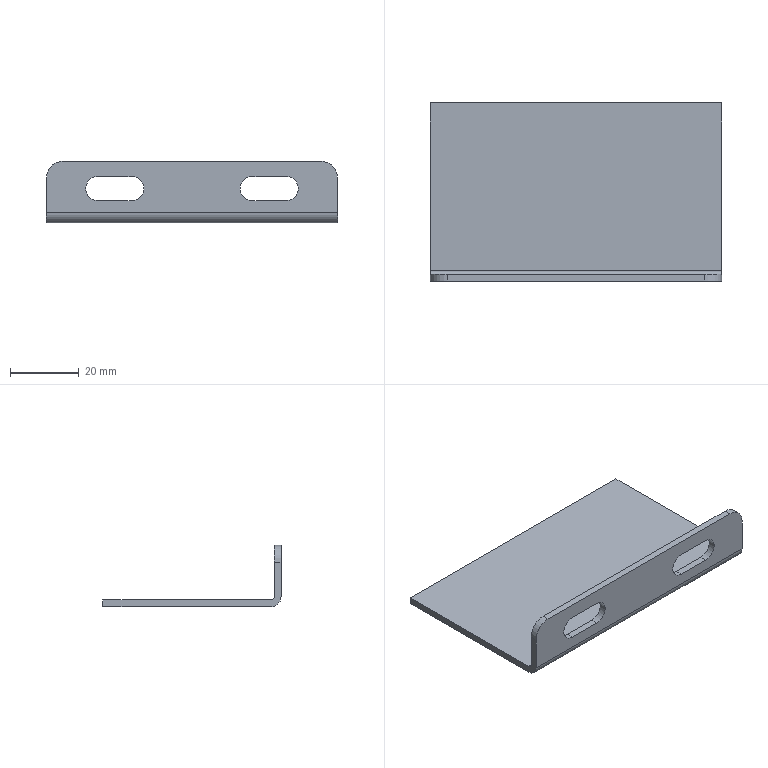Part | NX | features BLEND 2, DATUM_CSYS 2, EXTRUDE 2, SKETCH 2, EXTRACT_DATUM_PLANE 1 | 1 solid | 20 faces | box 85 x 52 x 18 mm | volume 10959 mm3 | plane 12 | cylinder 8 | commonest cylinder face diameters 7 x4 10 x2 2 x1 6 x1
STEP:
#1=CARTESIAN_POINT('',(-27.5,-27.,93.5));
#2=VERTEX_POINT('',#1);
#3=CARTESIAN_POINT('',(-27.5,-27.,100.5));
#4=VERTEX_POINT('',#3);
#5=CARTESIAN_POINT('',(-27.5,-27.,97.));
#6=DIRECTION('',(0.,1.,0.));
#7=DIRECTION('',(0.,0.,-1.));
#8=AXIS2_PLACEMENT_3D('',#5,#6,#7);
#9=CIRCLE('',#8,3.5);
#10=EDGE_CURVE('',#2,#4,#9,.T.);
#11=ORIENTED_EDGE('',*,*,#10,.T.);
#12=CARTESIAN_POINT('',(-17.5,-27.,100.5));
#13=VERTEX_POINT('',#12);
#14=CARTESIAN_POINT('',(-27.5,-27.,100.5));
#15=DIRECTION('',(1.,0.,0.));
#16=VECTOR('',#15,1000.);
#17=LINE('',#14,#16);
#18=EDGE_CURVE('',#4,#13,#17,.T.);
#19=ORIENTED_EDGE('',*,*,#18,.T.);
#20=CARTESIAN_POINT('',(-17.5,-27.,93.5));
#21=VERTEX_POINT('',#20);
#22=CARTESIAN_POINT('',(-17.5,-27.,97.));
#23=DIRECTION('',(0.,1.,0.));
#24=DIRECTION('',(0.,0.,1.));
#25=AXIS2_PLACEMENT_3D('',#22,#23,#24);
#26=CIRCLE('',#25,3.5);
#27=EDGE_CURVE('',#13,#21,#26,.T.);
#28=ORIENTED_EDGE('',*,*,#27,.T.);
#29=CARTESIAN_POINT('',(-17.5,-27.,93.5));
#30=DIRECTION('',(-1.,0.,0.));
#31=VECTOR('',#30,1000.);
#32=LINE('',#29,#31);
#33=EDGE_CURVE('',#21,#2,#32,.T.);
#34=ORIENTED_EDGE('',*,*,#33,.T.);
#35=EDGE_LOOP('',(#11,#19,#28,#34));
#36=FACE_BOUND('',#35,.T.);
#37=CARTESIAN_POINT('',(-37.5,-27.,105.));
#38=VERTEX_POINT('',#37);
#39=CARTESIAN_POINT('',(37.5,-27.,105.));
#40=VERTEX_POINT('',#39);
#41=CARTESIAN_POINT('',(-42.5,-27.,105.));
#42=DIRECTION('',(1.,0.,0.));
#43=VECTOR('',#42,1000.);
#44=LINE('',#41,#43);
#45=EDGE_CURVE('',#38,#40,#44,.T.);
#46=ORIENTED_EDGE('',*,*,#45,.F.);
#47=CARTESIAN_POINT('',(-42.5,-27.,100.));
#48=VERTEX_POINT('',#47);
#49=CARTESIAN_POINT('',(-37.5,-27.,100.));
#50=DIRECTION('',(0.,1.,0.));
#51=DIRECTION('',(0.,0.,1.));
#52=AXIS2_PLACEMENT_3D('',#49,#50,#51);
#53=CIRCLE('',#52,5.);
#54=EDGE_CURVE('',#38,#48,#53,.F.);
#55=ORIENTED_EDGE('',*,*,#54,.T.);
#56=CARTESIAN_POINT('',(-42.5,-27.,90.));
#57=VERTEX_POINT('',#56);
#58=CARTESIAN_POINT('',(-42.5,-27.,90.));
#59=DIRECTION('',(0.,0.,1.));
#60=VECTOR('',#59,1000.);
#61=LINE('',#58,#60);
#62=EDGE_CURVE('',#57,#48,#61,.T.);
#63=ORIENTED_EDGE('',*,*,#62,.F.);
#64=CARTESIAN_POINT('',(42.5,-27.,90.));
#65=VERTEX_POINT('',#64);
#66=CARTESIAN_POINT('',(-42.5,-27.,90.));
#67=DIRECTION('',(1.,0.,0.));
#68=VECTOR('',#67,1000.);
#69=LINE('',#66,#68);
#70=EDGE_CURVE('',#57,#65,#69,.T.);
#71=ORIENTED_EDGE('',*,*,#70,.T.);
#72=CARTESIAN_POINT('',(42.5,-27.,100.));
#73=VERTEX_POINT('',#72);
#74=CARTESIAN_POINT('',(42.5,-27.,100.));
#75=DIRECTION('',(0.,0.,1.));
#76=VECTOR('',#75,1000.);
#77=LINE('',#74,#76);
#78=EDGE_CURVE('',#65,#73,#77,.T.);
#79=ORIENTED_EDGE('',*,*,#78,.T.);
#80=CARTESIAN_POINT('',(37.5,-27.,100.));
#81=DIRECTION('',(0.,1.,0.));
#82=DIRECTION('',(0.,0.,1.));
#83=AXIS2_PLACEMENT_3D('',#80,#81,#82);
#84=CIRCLE('',#83,5.);
#85=EDGE_CURVE('',#73,#40,#84,.F.);
#86=ORIENTED_EDGE('',*,*,#85,.T.);
#87=EDGE_LOOP('',(#46,#55,#63,#71,#79,#86));
#88=FACE_BOUND('',#87,.T.);
#89=CARTESIAN_POINT('',(17.5,-27.,100.5));
#90=VERTEX_POINT('',#89);
#91=CARTESIAN_POINT('',(27.5,-27.,100.5));
#92=VERTEX_POINT('',#91);
#93=CARTESIAN_POINT('',(17.5,-27.,100.5));
#94=DIRECTION('',(1.,0.,0.));
#95=VECTOR('',#94,1000.);
#96=LINE('',#93,#95);
#97=EDGE_CURVE('',#90,#92,#96,.T.);
#98=ORIENTED_EDGE('',*,*,#97,.T.);
#99=CARTESIAN_POINT('',(27.5,-27.,93.5));
#100=VERTEX_POINT('',#99);
#101=CARTESIAN_POINT('',(27.5,-27.,97.));
#102=DIRECTION('',(0.,1.,0.));
#103=DIRECTION('',(0.,0.,1.));
#104=AXIS2_PLACEMENT_3D('',#101,#102,#103);
#105=CIRCLE('',#104,3.5);
#106=EDGE_CURVE('',#92,#100,#105,.T.);
#107=ORIENTED_EDGE('',*,*,#106,.T.);
#108=CARTESIAN_POINT('',(17.5,-27.,93.5));
#109=VERTEX_POINT('',#108);
#110=CARTESIAN_POINT('',(27.5,-27.,93.5));
#111=DIRECTION('',(-1.,0.,0.));
#112=VECTOR('',#111,1000.);
#113=LINE('',#110,#112);
#114=EDGE_CURVE('',#100,#109,#113,.T.);
#115=ORIENTED_EDGE('',*,*,#114,.T.);
#116=CARTESIAN_POINT('',(17.5,-27.,97.));
#117=DIRECTION('',(0.,1.,0.));
#118=DIRECTION('',(0.,0.,-1.));
#119=AXIS2_PLACEMENT_3D('',#116,#117,#118);
#120=CIRCLE('',#119,3.5);
#121=EDGE_CURVE('',#109,#90,#120,.T.);
#122=ORIENTED_EDGE('',*,*,#121,.T.);
#123=EDGE_LOOP('',(#98,#107,#115,#122));
#124=FACE_BOUND('',#123,.T.);
#125=CARTESIAN_POINT('',(-42.5,-27.,100.));
#126=DIRECTION('',(0.,1.,0.));
#127=DIRECTION('',(0.,0.,1.));
#128=AXIS2_PLACEMENT_3D('',#125,#126,#127);
#129=PLANE('',#128);
#130=ADVANCED_FACE('',(#36,#88,#124),#129,.F.);
#131=CARTESIAN_POINT('',(-27.5,-25.,93.5));
#132=VERTEX_POINT('',#131);
#133=CARTESIAN_POINT('',(-27.5,-25.,100.5));
#134=VERTEX_POINT('',#133);
#135=CARTESIAN_POINT('',(-27.5,-25.,97.));
#136=DIRECTION('',(0.,-1.,0.));
#137=DIRECTION('',(0.,0.,-1.));
#138=AXIS2_PLACEMENT_3D('',#135,#136,#137);
#139=CIRCLE('',#138,3.5);
#140=EDGE_CURVE('',#132,#134,#139,.F.);
#141=ORIENTED_EDGE('',*,*,#140,.F.);
#142=CARTESIAN_POINT('',(-17.5,-25.,93.5));
#143=VERTEX_POINT('',#142);
#144=CARTESIAN_POINT('',(-42.5,-25.,93.5));
#145=DIRECTION('',(-1.,0.,0.));
#146=VECTOR('',#145,1000.);
#147=LINE('',#144,#146);
#148=EDGE_CURVE('',#143,#132,#147,.T.);
#149=ORIENTED_EDGE('',*,*,#148,.F.);
#150=CARTESIAN_POINT('',(-17.5,-25.,100.5));
#151=VERTEX_POINT('',#150);
#152=CARTESIAN_POINT('',(-17.5,-25.,97.));
#153=DIRECTION('',(0.,-1.,0.));
#154=DIRECTION('',(0.,0.,-1.));
#155=AXIS2_PLACEMENT_3D('',#152,#153,#154);
#156=CIRCLE('',#155,3.5);
#157=EDGE_CURVE('',#151,#143,#156,.F.);
#158=ORIENTED_EDGE('',*,*,#157,.F.);
#159=CARTESIAN_POINT('',(-42.5,-25.,100.5));
#160=DIRECTION('',(1.,0.,0.));
#161=VECTOR('',#160,1000.);
#162=LINE('',#159,#161);
#163=EDGE_CURVE('',#134,#151,#162,.T.);
#164=ORIENTED_EDGE('',*,*,#163,.F.);
#165=EDGE_LOOP('',(#141,#149,#158,#164));
#166=FACE_BOUND('',#165,.T.);
#167=CARTESIAN_POINT('',(-42.5,-25.,100.));
#168=VERTEX_POINT('',#167);
#169=CARTESIAN_POINT('',(-42.5,-25.,90.));
#170=VERTEX_POINT('',#169);
#171=CARTESIAN_POINT('',(-42.5,-25.,105.));
#172=DIRECTION('',(0.,0.,-1.));
#173=VECTOR('',#172,1000.);
#174=LINE('',#171,#173);
#175=EDGE_CURVE('',#168,#170,#174,.T.);
#176=ORIENTED_EDGE('',*,*,#175,.F.);
#177=CARTESIAN_POINT('',(-37.5,-25.,105.));
#178=VERTEX_POINT('',#177);
#179=CARTESIAN_POINT('',(-37.5,-25.,100.));
#180=DIRECTION('',(0.,-1.,0.));
#181=DIRECTION('',(0.,0.,-1.));
#182=AXIS2_PLACEMENT_3D('',#179,#180,#181);
#183=CIRCLE('',#182,5.);
#184=EDGE_CURVE('',#168,#178,#183,.F.);
#185=ORIENTED_EDGE('',*,*,#184,.T.);
#186=CARTESIAN_POINT('',(37.5,-25.,105.));
#187=VERTEX_POINT('',#186);
#188=CARTESIAN_POINT('',(-42.5,-25.,105.));
#189=DIRECTION('',(1.,0.,0.));
#190=VECTOR('',#189,1000.);
#191=LINE('',#188,#190);
#192=EDGE_CURVE('',#178,#187,#191,.T.);
#193=ORIENTED_EDGE('',*,*,#192,.T.);
#194=CARTESIAN_POINT('',(42.5,-25.,100.));
#195=VERTEX_POINT('',#194);
#196=CARTESIAN_POINT('',(37.5,-25.,100.));
#197=DIRECTION('',(0.,-1.,0.));
#198=DIRECTION('',(0.,0.,-1.));
#199=AXIS2_PLACEMENT_3D('',#196,#197,#198);
#200=CIRCLE('',#199,5.);
#201=EDGE_CURVE('',#187,#195,#200,.F.);
#202=ORIENTED_EDGE('',*,*,#201,.T.);
#203=CARTESIAN_POINT('',(42.5,-25.,90.));
#204=VERTEX_POINT('',#203);
#205=CARTESIAN_POINT('',(42.5,-25.,100.));
#206=DIRECTION('',(0.,0.,-1.));
#207=VECTOR('',#206,1000.);
#208=LINE('',#205,#207);
#209=EDGE_CURVE('',#195,#204,#208,.T.);
#210=ORIENTED_EDGE('',*,*,#209,.T.);
#211=CARTESIAN_POINT('',(-42.5,-25.,90.));
#212=DIRECTION('',(1.,0.,0.));
#213=VECTOR('',#212,1000.);
#214=LINE('',#211,#213);
#215=EDGE_CURVE('',#170,#204,#214,.T.);
#216=ORIENTED_EDGE('',*,*,#215,.F.);
#217=EDGE_LOOP('',(#176,#185,#193,#202,#210,#216));
#218=FACE_BOUND('',#217,.T.);
#219=CARTESIAN_POINT('',(17.5,-25.,100.5));
#220=VERTEX_POINT('',#219);
#221=CARTESIAN_POINT('',(27.5,-25.,100.5));
#222=VERTEX_POINT('',#221);
#223=CARTESIAN_POINT('',(-42.5,-25.,100.5));
#224=DIRECTION('',(1.,0.,0.));
#225=VECTOR('',#224,1000.);
#226=LINE('',#223,#225);
#227=EDGE_CURVE('',#220,#222,#226,.T.);
#228=ORIENTED_EDGE('',*,*,#227,.F.);
#229=CARTESIAN_POINT('',(17.5,-25.,93.5));
#230=VERTEX_POINT('',#229);
#231=CARTESIAN_POINT('',(17.5,-25.,97.));
#232=DIRECTION('',(0.,-1.,0.));
#233=DIRECTION('',(0.,0.,-1.));
#234=AXIS2_PLACEMENT_3D('',#231,#232,#233);
#235=CIRCLE('',#234,3.5);
#236=EDGE_CURVE('',#230,#220,#235,.F.);
#237=ORIENTED_EDGE('',*,*,#236,.F.);
#238=CARTESIAN_POINT('',(27.5,-25.,93.5));
#239=VERTEX_POINT('',#238);
#240=CARTESIAN_POINT('',(-42.5,-25.,93.5));
#241=DIRECTION('',(-1.,0.,0.));
#242=VECTOR('',#241,1000.);
#243=LINE('',#240,#242);
#244=EDGE_CURVE('',#239,#230,#243,.T.);
#245=ORIENTED_EDGE('',*,*,#244,.F.);
#246=CARTESIAN_POINT('',(27.5,-25.,97.));
#247=DIRECTION('',(0.,-1.,0.));
#248=DIRECTION('',(0.,0.,-1.));
#249=AXIS2_PLACEMENT_3D('',#246,#247,#248);
#250=CIRCLE('',#249,3.5);
#251=EDGE_CURVE('',#222,#239,#250,.F.);
#252=ORIENTED_EDGE('',*,*,#251,.F.);
#253=EDGE_LOOP('',(#228,#237,#245,#252));
#254=FACE_BOUND('',#253,.T.);
#255=CARTESIAN_POINT('',(-42.5,-25.,100.));
#256=DIRECTION('',(0.,-1.,0.));
#257=DIRECTION('',(0.,0.,-1.));
#258=AXIS2_PLACEMENT_3D('',#255,#256,#257);
#259=PLANE('',#258);
#260=ADVANCED_FACE('',(#166,#218,#254),#259,.F.);
#261=ORIENTED_EDGE('',*,*,#192,.F.);
#262=CARTESIAN_POINT('',(-37.5,-27.,105.));
#263=DIRECTION('',(0.,1.,0.));
#264=VECTOR('',#263,1000.);
#265=LINE('',#262,#264);
#266=EDGE_CURVE('',#178,#38,#265,.F.);
#267=ORIENTED_EDGE('',*,*,#266,.T.);
#268=ORIENTED_EDGE('',*,*,#45,.T.);
#269=CARTESIAN_POINT('',(37.5,-25.,105.));
#270=DIRECTION('',(0.,1.,0.));
#271=VECTOR('',#270,1000.);
#272=LINE('',#269,#271);
#273=EDGE_CURVE('',#40,#187,#272,.T.);
#274=ORIENTED_EDGE('',*,*,#273,.T.);
#275=EDGE_LOOP('',(#261,#267,#268,#274));
#276=FACE_BOUND('',#275,.T.);
#277=CARTESIAN_POINT('',(-42.5,-27.,105.));
#278=DIRECTION('',(0.,0.,-1.));
#279=DIRECTION('',(-1.,0.,0.));
#280=AXIS2_PLACEMENT_3D('',#277,#278,#279);
#281=PLANE('',#280);
#282=ADVANCED_FACE('',(#276),#281,.F.);
#283=CARTESIAN_POINT('',(42.5,-24.,89.));
#284=VERTEX_POINT('',#283);
#285=CARTESIAN_POINT('',(42.5,-24.,90.));
#286=DIRECTION('',(1.,0.,0.));
#287=DIRECTION('',(0.,0.,-1.));
#288=AXIS2_PLACEMENT_3D('',#285,#286,#287);
#289=CIRCLE('',#288,1.);
#290=EDGE_CURVE('',#204,#284,#289,.T.);
#291=ORIENTED_EDGE('',*,*,#290,.T.);
#292=CARTESIAN_POINT('',(-42.5,-24.,89.));
#293=VERTEX_POINT('',#292);
#294=CARTESIAN_POINT('',(-42.5,-24.,89.));
#295=DIRECTION('',(1.,0.,0.));
#296=VECTOR('',#295,1000.);
#297=LINE('',#294,#296);
#298=EDGE_CURVE('',#293,#284,#297,.T.);
#299=ORIENTED_EDGE('',*,*,#298,.F.);
#300=CARTESIAN_POINT('',(-42.5,-24.,90.));
#301=DIRECTION('',(1.,0.,0.));
#302=DIRECTION('',(0.,0.,-1.));
#303=AXIS2_PLACEMENT_3D('',#300,#301,#302);
#304=CIRCLE('',#303,1.);
#305=EDGE_CURVE('',#170,#293,#304,.T.);
#306=ORIENTED_EDGE('',*,*,#305,.F.);
#307=ORIENTED_EDGE('',*,*,#215,.T.);
#308=EDGE_LOOP('',(#291,#299,#306,#307));
#309=FACE_BOUND('',#308,.T.);
#310=CARTESIAN_POINT('',(-42.5,-24.,90.));
#311=DIRECTION('',(1.,0.,0.));
#312=DIRECTION('',(0.,0.,-1.));
#313=AXIS2_PLACEMENT_3D('',#310,#311,#312);
#314=CYLINDRICAL_SURFACE('',#313,1.);
#315=ADVANCED_FACE('',(#309),#314,.F.);
#316=CARTESIAN_POINT('',(42.5,25.,89.));
#317=VERTEX_POINT('',#316);
#318=CARTESIAN_POINT('',(42.5,24.,89.));
#319=DIRECTION('',(0.,1.,0.));
#320=VECTOR('',#319,1000.);
#321=LINE('',#318,#320);
#322=EDGE_CURVE('',#284,#317,#321,.T.);
#323=ORIENTED_EDGE('',*,*,#322,.T.);
#324=CARTESIAN_POINT('',(-42.5,25.,89.));
#325=VERTEX_POINT('',#324);
#326=CARTESIAN_POINT('',(-42.5,25.,89.));
#327=DIRECTION('',(1.,0.,0.));
#328=VECTOR('',#327,1000.);
#329=LINE('',#326,#328);
#330=EDGE_CURVE('',#325,#317,#329,.T.);
#331=ORIENTED_EDGE('',*,*,#330,.F.);
#332=CARTESIAN_POINT('',(-42.5,-24.,89.));
#333=DIRECTION('',(0.,1.,0.));
#334=VECTOR('',#333,1000.);
#335=LINE('',#332,#334);
#336=EDGE_CURVE('',#293,#325,#335,.T.);
#337=ORIENTED_EDGE('',*,*,#336,.F.);
#338=ORIENTED_EDGE('',*,*,#298,.T.);
#339=EDGE_LOOP('',(#323,#331,#337,#338));
#340=FACE_BOUND('',#339,.T.);
#341=CARTESIAN_POINT('',(-42.5,24.,89.));
#342=DIRECTION('',(0.,0.,-1.));
#343=DIRECTION('',(-1.,0.,0.));
#344=AXIS2_PLACEMENT_3D('',#341,#342,#343);
#345=PLANE('',#344);
#346=ADVANCED_FACE('',(#340),#345,.F.);
#347=CARTESIAN_POINT('',(42.5,25.,87.));
#348=VERTEX_POINT('',#347);
#349=CARTESIAN_POINT('',(42.5,25.,89.));
#350=DIRECTION('',(0.,0.,-1.));
#351=VECTOR('',#350,1000.);
#352=LINE('',#349,#351);
#353=EDGE_CURVE('',#317,#348,#352,.T.);
#354=ORIENTED_EDGE('',*,*,#353,.T.);
#355=CARTESIAN_POINT('',(-42.5,25.,87.));
#356=VERTEX_POINT('',#355);
#357=CARTESIAN_POINT('',(-42.5,25.,87.));
#358=DIRECTION('',(1.,0.,0.));
#359=VECTOR('',#358,1000.);
#360=LINE('',#357,#359);
#361=EDGE_CURVE('',#356,#348,#360,.T.);
#362=ORIENTED_EDGE('',*,*,#361,.F.);
#363=CARTESIAN_POINT('',(-42.5,25.,89.));
#364=DIRECTION('',(0.,0.,-1.));
#365=VECTOR('',#364,1000.);
#366=LINE('',#363,#365);
#367=EDGE_CURVE('',#325,#356,#366,.T.);
#368=ORIENTED_EDGE('',*,*,#367,.F.);
#369=ORIENTED_EDGE('',*,*,#330,.T.);
#370=EDGE_LOOP('',(#354,#362,#368,#369));
#371=FACE_BOUND('',#370,.T.);
#372=CARTESIAN_POINT('',(-42.5,25.,89.));
#373=DIRECTION('',(0.,-1.,0.));
#374=DIRECTION('',(0.,0.,-1.));
#375=AXIS2_PLACEMENT_3D('',#372,#373,#374);
#376=PLANE('',#375);
#377=ADVANCED_FACE('',(#371),#376,.F.);
#378=CARTESIAN_POINT('',(42.5,-24.,87.));
#379=VERTEX_POINT('',#378);
#380=CARTESIAN_POINT('',(42.5,24.,87.));
#381=DIRECTION('',(0.,-1.,0.));
#382=VECTOR('',#381,1000.);
#383=LINE('',#380,#382);
#384=EDGE_CURVE('',#348,#379,#383,.T.);
#385=ORIENTED_EDGE('',*,*,#384,.T.);
#386=CARTESIAN_POINT('',(-42.5,-24.,87.));
#387=VERTEX_POINT('',#386);
#388=CARTESIAN_POINT('',(-42.5,-24.,87.));
#389=DIRECTION('',(1.,0.,0.));
#390=VECTOR('',#389,1000.);
#391=LINE('',#388,#390);
#392=EDGE_CURVE('',#387,#379,#391,.T.);
#393=ORIENTED_EDGE('',*,*,#392,.F.);
#394=CARTESIAN_POINT('',(-42.5,25.,87.));
#395=DIRECTION('',(0.,-1.,0.));
#396=VECTOR('',#395,1000.);
#397=LINE('',#394,#396);
#398=EDGE_CURVE('',#356,#387,#397,.T.);
#399=ORIENTED_EDGE('',*,*,#398,.F.);
#400=ORIENTED_EDGE('',*,*,#361,.T.);
#401=EDGE_LOOP('',(#385,#393,#399,#400));
#402=FACE_BOUND('',#401,.T.);
#403=CARTESIAN_POINT('',(-42.5,24.,87.));
#404=DIRECTION('',(0.,0.,1.));
#405=DIRECTION('',(1.,0.,0.));
#406=AXIS2_PLACEMENT_3D('',#403,#404,#405);
#407=PLANE('',#406);
#408=ADVANCED_FACE('',(#402),#407,.F.);
#409=CARTESIAN_POINT('',(42.5,-24.,90.));
#410=DIRECTION('',(-1.,0.,0.));
#411=DIRECTION('',(0.,-1.,0.));
#412=AXIS2_PLACEMENT_3D('',#409,#410,#411);
#413=CIRCLE('',#412,3.);
#414=EDGE_CURVE('',#379,#65,#413,.T.);
#415=ORIENTED_EDGE('',*,*,#414,.T.);
#416=ORIENTED_EDGE('',*,*,#70,.F.);
#417=CARTESIAN_POINT('',(-42.5,-24.,90.));
#418=DIRECTION('',(-1.,0.,0.));
#419=DIRECTION('',(0.,-1.,0.));
#420=AXIS2_PLACEMENT_3D('',#417,#418,#419);
#421=CIRCLE('',#420,3.);
#422=EDGE_CURVE('',#387,#57,#421,.T.);
#423=ORIENTED_EDGE('',*,*,#422,.F.);
#424=ORIENTED_EDGE('',*,*,#392,.T.);
#425=EDGE_LOOP('',(#415,#416,#423,#424));
#426=FACE_BOUND('',#425,.T.);
#427=CARTESIAN_POINT('',(-42.5,-24.,90.));
#428=DIRECTION('',(1.,0.,0.));
#429=DIRECTION('',(0.,0.,-1.));
#430=AXIS2_PLACEMENT_3D('',#427,#428,#429);
#431=CYLINDRICAL_SURFACE('',#430,3.);
#432=ADVANCED_FACE('',(#426),#431,.T.);
#433=ORIENTED_EDGE('',*,*,#62,.T.);
#434=CARTESIAN_POINT('',(-42.5,-24.,100.));
#435=DIRECTION('',(0.,1.,0.));
#436=VECTOR('',#435,1000.);
#437=LINE('',#434,#436);
#438=EDGE_CURVE('',#48,#168,#437,.T.);
#439=ORIENTED_EDGE('',*,*,#438,.T.);
#440=ORIENTED_EDGE('',*,*,#175,.T.);
#441=ORIENTED_EDGE('',*,*,#305,.T.);
#442=ORIENTED_EDGE('',*,*,#336,.T.);
#443=ORIENTED_EDGE('',*,*,#367,.T.);
#444=ORIENTED_EDGE('',*,*,#398,.T.);
#445=ORIENTED_EDGE('',*,*,#422,.T.);
#446=EDGE_LOOP('',(#433,#439,#440,#441,#442,#443,#444,#445));
#447=FACE_BOUND('',#446,.T.);
#448=CARTESIAN_POINT('',(-42.5,-24.,90.));
#449=DIRECTION('',(1.,0.,0.));
#450=DIRECTION('',(0.,0.,-1.));
#451=AXIS2_PLACEMENT_3D('',#448,#449,#450);
#452=PLANE('',#451);
#453=ADVANCED_FACE('',(#447),#452,.F.);
#454=ORIENTED_EDGE('',*,*,#209,.F.);
#455=CARTESIAN_POINT('',(42.5,-27.,100.));
#456=DIRECTION('',(0.,1.,0.));
#457=VECTOR('',#456,1000.);
#458=LINE('',#455,#457);
#459=EDGE_CURVE('',#195,#73,#458,.F.);
#460=ORIENTED_EDGE('',*,*,#459,.T.);
#461=ORIENTED_EDGE('',*,*,#78,.F.);
#462=ORIENTED_EDGE('',*,*,#414,.F.);
#463=ORIENTED_EDGE('',*,*,#384,.F.);
#464=ORIENTED_EDGE('',*,*,#353,.F.);
#465=ORIENTED_EDGE('',*,*,#322,.F.);
#466=ORIENTED_EDGE('',*,*,#290,.F.);
#467=EDGE_LOOP('',(#454,#460,#461,#462,#463,#464,#465,#466));
#468=FACE_BOUND('',#467,.T.);
#469=CARTESIAN_POINT('',(42.5,-24.,90.));
#470=DIRECTION('',(1.,0.,0.));
#471=DIRECTION('',(0.,0.,-1.));
#472=AXIS2_PLACEMENT_3D('',#469,#470,#471);
#473=PLANE('',#472);
#474=ADVANCED_FACE('',(#468),#473,.T.);
#475=ORIENTED_EDGE('',*,*,#85,.F.);
#476=ORIENTED_EDGE('',*,*,#459,.F.);
#477=ORIENTED_EDGE('',*,*,#201,.F.);
#478=ORIENTED_EDGE('',*,*,#273,.F.);
#479=EDGE_LOOP('',(#475,#476,#477,#478));
#480=FACE_BOUND('',#479,.T.);
#481=CARTESIAN_POINT('',(37.5,-27.,100.));
#482=DIRECTION('',(0.,-1.,0.));
#483=DIRECTION('',(0.,0.,-1.));
#484=AXIS2_PLACEMENT_3D('',#481,#482,#483);
#485=CYLINDRICAL_SURFACE('',#484,5.);
#486=ADVANCED_FACE('',(#480),#485,.T.);
#487=ORIENTED_EDGE('',*,*,#54,.F.);
#488=ORIENTED_EDGE('',*,*,#266,.F.);
#489=ORIENTED_EDGE('',*,*,#184,.F.);
#490=ORIENTED_EDGE('',*,*,#438,.F.);
#491=EDGE_LOOP('',(#487,#488,#489,#490));
#492=FACE_BOUND('',#491,.T.);
#493=CARTESIAN_POINT('',(-37.5,-24.,100.));
#494=DIRECTION('',(0.,1.,0.));
#495=DIRECTION('',(0.,0.,1.));
#496=AXIS2_PLACEMENT_3D('',#493,#494,#495);
#497=CYLINDRICAL_SURFACE('',#496,5.);
#498=ADVANCED_FACE('',(#492),#497,.T.);
#499=ORIENTED_EDGE('',*,*,#140,.T.);
#500=CARTESIAN_POINT('',(-27.5,425.,100.5));
#501=DIRECTION('',(0.,-1.,0.));
#502=VECTOR('',#501,1000.);
#503=LINE('',#500,#502);
#504=EDGE_CURVE('',#4,#134,#503,.F.);
#505=ORIENTED_EDGE('',*,*,#504,.F.);
#506=ORIENTED_EDGE('',*,*,#10,.F.);
#507=CARTESIAN_POINT('',(-27.5,425.,93.5));
#508=DIRECTION('',(0.,-1.,0.));
#509=VECTOR('',#508,1000.);
#510=LINE('',#507,#509);
#511=EDGE_CURVE('',#2,#132,#510,.F.);
#512=ORIENTED_EDGE('',*,*,#511,.T.);
#513=EDGE_LOOP('',(#499,#505,#506,#512));
#514=FACE_BOUND('',#513,.T.);
#515=CARTESIAN_POINT('',(-27.5,425.,97.));
#516=DIRECTION('',(0.,-1.,0.));
#517=DIRECTION('',(0.,0.,-1.));
#518=AXIS2_PLACEMENT_3D('',#515,#516,#517);
#519=CYLINDRICAL_SURFACE('',#518,3.5);
#520=ADVANCED_FACE('',(#514),#519,.F.);
#521=ORIENTED_EDGE('',*,*,#163,.T.);
#522=CARTESIAN_POINT('',(-17.5,425.,100.5));
#523=DIRECTION('',(0.,-1.,0.));
#524=VECTOR('',#523,1000.);
#525=LINE('',#522,#524);
#526=EDGE_CURVE('',#13,#151,#525,.F.);
#527=ORIENTED_EDGE('',*,*,#526,.F.);
#528=ORIENTED_EDGE('',*,*,#18,.F.);
#529=ORIENTED_EDGE('',*,*,#504,.T.);
#530=EDGE_LOOP('',(#521,#527,#528,#529));
#531=FACE_BOUND('',#530,.T.);
#532=CARTESIAN_POINT('',(-27.5,425.,100.5));
#533=DIRECTION('',(0.,0.,-1.));
#534=DIRECTION('',(-1.,0.,0.));
#535=AXIS2_PLACEMENT_3D('',#532,#533,#534);
#536=PLANE('',#535);
#537=ADVANCED_FACE('',(#531),#536,.T.);
#538=ORIENTED_EDGE('',*,*,#157,.T.);
#539=CARTESIAN_POINT('',(-17.5,425.,93.5));
#540=DIRECTION('',(0.,-1.,0.));
#541=VECTOR('',#540,1000.);
#542=LINE('',#539,#541);
#543=EDGE_CURVE('',#21,#143,#542,.F.);
#544=ORIENTED_EDGE('',*,*,#543,.F.);
#545=ORIENTED_EDGE('',*,*,#27,.F.);
#546=ORIENTED_EDGE('',*,*,#526,.T.);
#547=EDGE_LOOP('',(#538,#544,#545,#546));
#548=FACE_BOUND('',#547,.T.);
#549=CARTESIAN_POINT('',(-17.5,425.,97.));
#550=DIRECTION('',(0.,-1.,0.));
#551=DIRECTION('',(0.,0.,-1.));
#552=AXIS2_PLACEMENT_3D('',#549,#550,#551);
#553=CYLINDRICAL_SURFACE('',#552,3.5);
#554=ADVANCED_FACE('',(#548),#553,.F.);
#555=ORIENTED_EDGE('',*,*,#148,.T.);
#556=ORIENTED_EDGE('',*,*,#511,.F.);
#557=ORIENTED_EDGE('',*,*,#33,.F.);
#558=ORIENTED_EDGE('',*,*,#543,.T.);
#559=EDGE_LOOP('',(#555,#556,#557,#558));
#560=FACE_BOUND('',#559,.T.);
#561=CARTESIAN_POINT('',(-17.5,425.,93.5));
#562=DIRECTION('',(0.,0.,1.));
#563=DIRECTION('',(1.,0.,0.));
#564=AXIS2_PLACEMENT_3D('',#561,#562,#563);
#565=PLANE('',#564);
#566=ADVANCED_FACE('',(#560),#565,.T.);
#567=ORIENTED_EDGE('',*,*,#227,.T.);
#568=CARTESIAN_POINT('',(27.5,425.,100.5));
#569=DIRECTION('',(0.,-1.,0.));
#570=VECTOR('',#569,1000.);
#571=LINE('',#568,#570);
#572=EDGE_CURVE('',#92,#222,#571,.F.);
#573=ORIENTED_EDGE('',*,*,#572,.F.);
#574=ORIENTED_EDGE('',*,*,#97,.F.);
#575=CARTESIAN_POINT('',(17.5,425.,100.5));
#576=DIRECTION('',(0.,-1.,0.));
#577=VECTOR('',#576,1000.);
#578=LINE('',#575,#577);
#579=EDGE_CURVE('',#90,#220,#578,.F.);
#580=ORIENTED_EDGE('',*,*,#579,.T.);
#581=EDGE_LOOP('',(#567,#573,#574,#580));
#582=FACE_BOUND('',#581,.T.);
#583=CARTESIAN_POINT('',(17.5,425.,100.5));
#584=DIRECTION('',(0.,0.,-1.));
#585=DIRECTION('',(-1.,0.,0.));
#586=AXIS2_PLACEMENT_3D('',#583,#584,#585);
#587=PLANE('',#586);
#588=ADVANCED_FACE('',(#582),#587,.T.);
#589=ORIENTED_EDGE('',*,*,#251,.T.);
#590=CARTESIAN_POINT('',(27.5,425.,93.5));
#591=DIRECTION('',(0.,-1.,0.));
#592=VECTOR('',#591,1000.);
#593=LINE('',#590,#592);
#594=EDGE_CURVE('',#100,#239,#593,.F.);
#595=ORIENTED_EDGE('',*,*,#594,.F.);
#596=ORIENTED_EDGE('',*,*,#106,.F.);
#597=ORIENTED_EDGE('',*,*,#572,.T.);
#598=EDGE_LOOP('',(#589,#595,#596,#597));
#599=FACE_BOUND('',#598,.T.);
#600=CARTESIAN_POINT('',(27.5,425.,97.));
#601=DIRECTION('',(0.,-1.,0.));
#602=DIRECTION('',(0.,0.,-1.));
#603=AXIS2_PLACEMENT_3D('',#600,#601,#602);
#604=CYLINDRICAL_SURFACE('',#603,3.5);
#605=ADVANCED_FACE('',(#599),#604,.F.);
#606=ORIENTED_EDGE('',*,*,#244,.T.);
#607=CARTESIAN_POINT('',(17.5,425.,93.5));
#608=DIRECTION('',(0.,-1.,0.));
#609=VECTOR('',#608,1000.);
#610=LINE('',#607,#609);
#611=EDGE_CURVE('',#109,#230,#610,.F.);
#612=ORIENTED_EDGE('',*,*,#611,.F.);
#613=ORIENTED_EDGE('',*,*,#114,.F.);
#614=ORIENTED_EDGE('',*,*,#594,.T.);
#615=EDGE_LOOP('',(#606,#612,#613,#614));
#616=FACE_BOUND('',#615,.T.);
#617=CARTESIAN_POINT('',(27.5,425.,93.5));
#618=DIRECTION('',(0.,0.,1.));
#619=DIRECTION('',(1.,0.,0.));
#620=AXIS2_PLACEMENT_3D('',#617,#618,#619);
#621=PLANE('',#620);
#622=ADVANCED_FACE('',(#616),#621,.T.);
#623=ORIENTED_EDGE('',*,*,#236,.T.);
#624=ORIENTED_EDGE('',*,*,#579,.F.);
#625=ORIENTED_EDGE('',*,*,#121,.F.);
#626=ORIENTED_EDGE('',*,*,#611,.T.);
#627=EDGE_LOOP('',(#623,#624,#625,#626));
#628=FACE_BOUND('',#627,.T.);
#629=CARTESIAN_POINT('',(17.5,425.,97.));
#630=DIRECTION('',(0.,-1.,0.));
#631=DIRECTION('',(0.,0.,-1.));
#632=AXIS2_PLACEMENT_3D('',#629,#630,#631);
#633=CYLINDRICAL_SURFACE('',#632,3.5);
#634=ADVANCED_FACE('',(#628),#633,.F.);
#635=CLOSED_SHELL('',(#130,#260,#282,#315,#346,#377,#408,#432,#453,#474,#486,#498,#520,#537,#554,#566,#588,#605,#622,#634));
#636=MANIFOLD_SOLID_BREP('',#635);
#637=(LENGTH_UNIT()NAMED_UNIT(*)SI_UNIT(.MILLI.,.METRE.));
#638=UNCERTAINTY_MEASURE_WITH_UNIT(LENGTH_MEASURE(0.00001),#637,'','');
#639=(NAMED_UNIT(*)PLANE_ANGLE_UNIT()SI_UNIT($,.RADIAN.));
#640=(NAMED_UNIT(*)SI_UNIT($,.STERADIAN.)SOLID_ANGLE_UNIT());
#641=(GEOMETRIC_REPRESENTATION_CONTEXT(3)GLOBAL_UNCERTAINTY_ASSIGNED_CONTEXT((#638))GLOBAL_UNIT_ASSIGNED_CONTEXT((#637,#639,#640))REPRESENTATION_CONTEXT('',''));
#642=ADVANCED_BREP_SHAPE_REPRESENTATION('',(#636),#641);